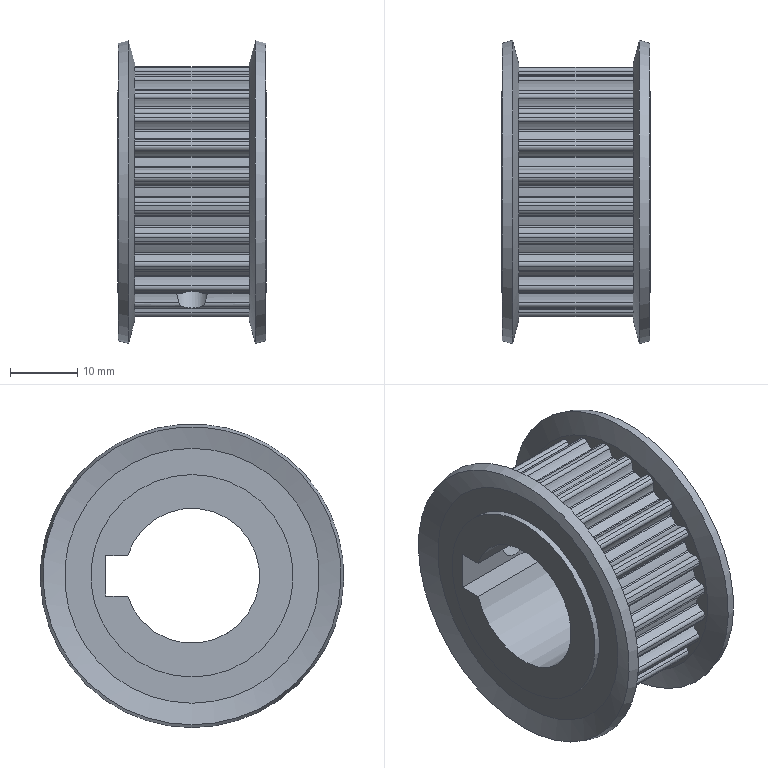Part | NX | features 5003_017_C-HTPA24S5M150-A-N20 2 | 1 solid | 226 faces | box 22 x 45 x 45 mm | volume 15371 mm3 | cylinder 211 | plane 9 | cone 6 | commonest cylinder face diameters 0.5 x52 1.1 x52 6.55 x52 33.7 x26 37.24 x24 4.92 x2